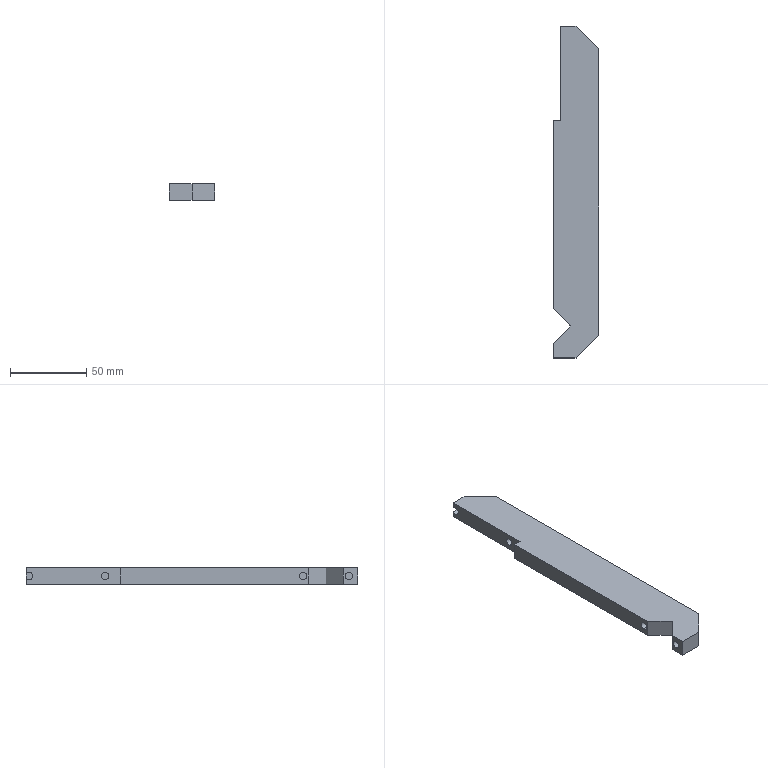Part | STEP file | CLAMP.ARM.1.stp | 1 solid | 25 faces | box 30 x 218 x 11 mm | volume 63871 mm3 | plane 16 | spline 5 | cylinder 4 | commonest cylinder face diameters 5 x4